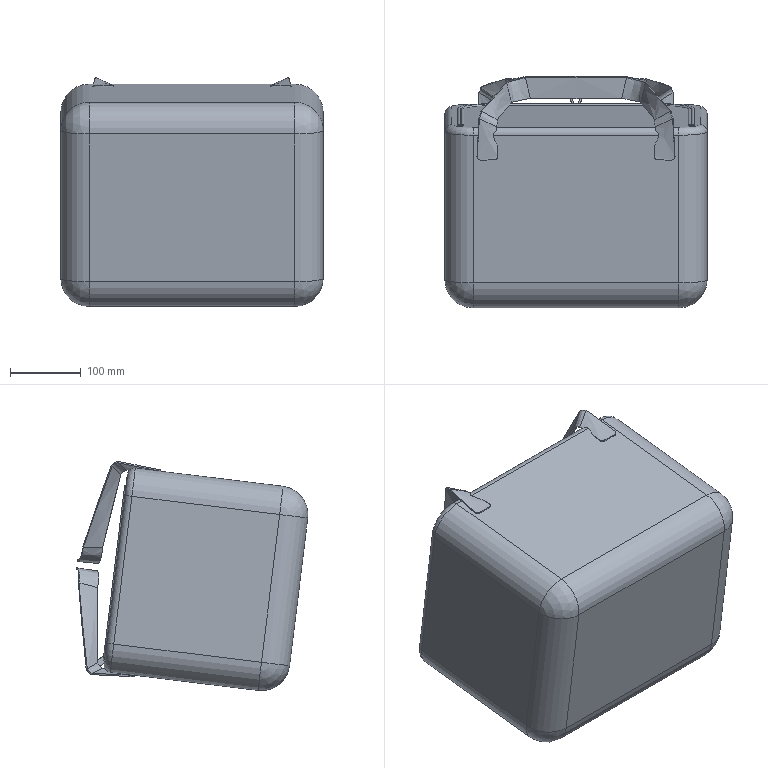Part | SolidWorks | features BaseBody 1 | 1 solid | 216 faces | box 370 x 327.003 x 323.13 mm | volume 1077655 mm3 | spline 104 | cylinder 50 | plane 38 | torus 16 | sphere 8 | commonest cylinder face diameters 4 x16 76 x8 80 x8 7 x6 9 x4 16 x4